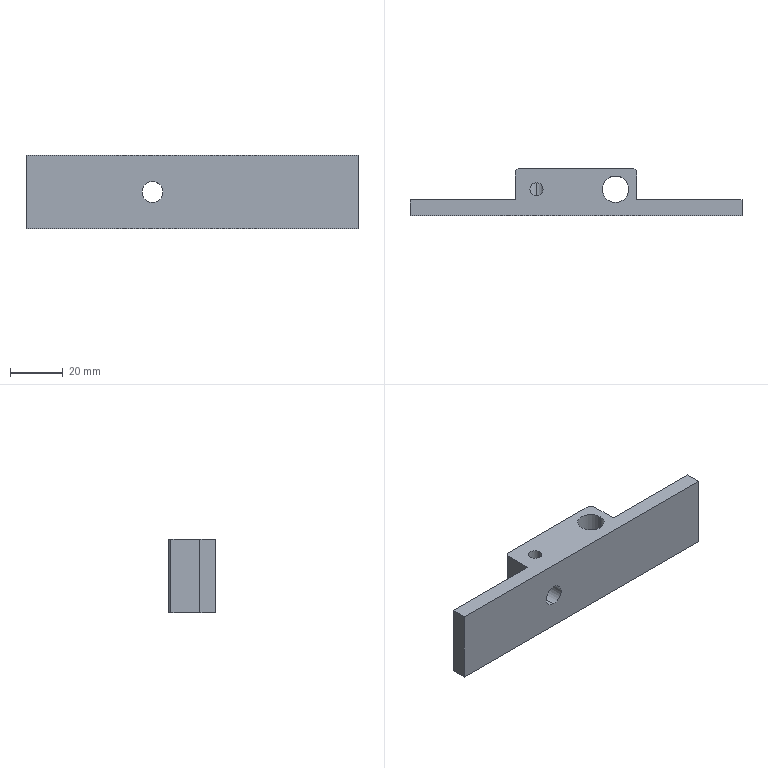Part | STEP file | BU-C01 | 1 solid | 22 faces | box 126 x 18 x 28 mm | volume 33069 mm3 | plane 14 | cylinder 8 | commonest cylinder face diameters 5 x4 8 x2 10 x2